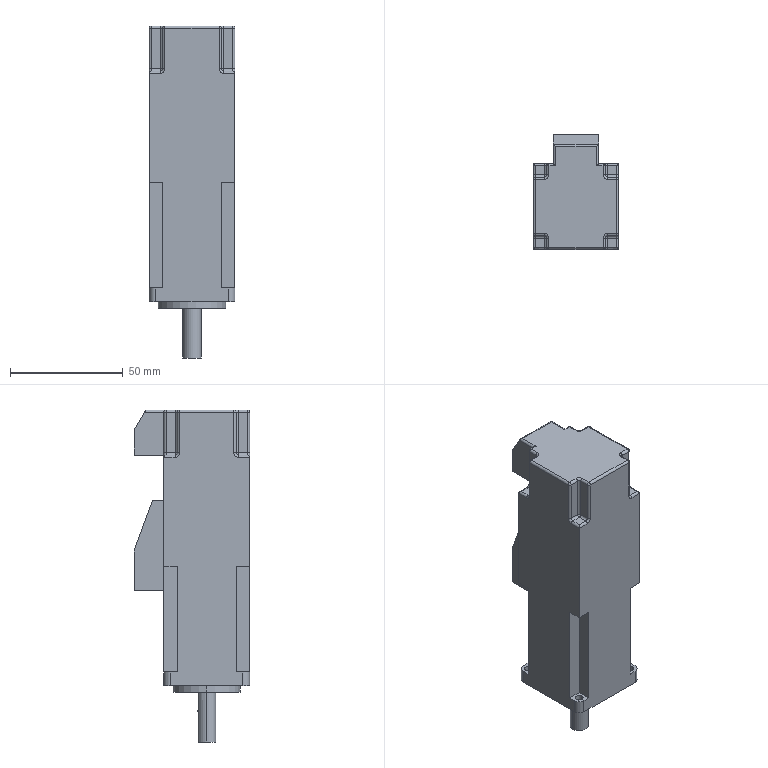Part | NX | features BREP 1 | 1 solid | 142 faces | box 38 x 51 x 147 mm | volume 181104 mm3 | cylinder 65 | plane 51 | torus 12 | sphere 12 | cone 2 | commonest cylinder face diameters 2 x44 3.4 x8 6 x4 2.5 x2 8 x2 28 x2